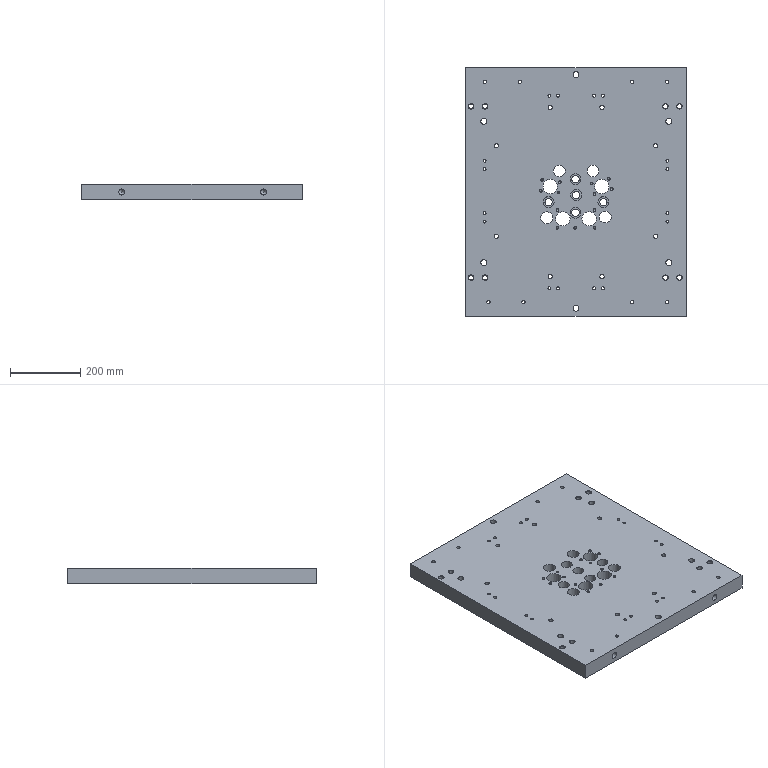Part | NX | features solid 2 | 1 solid | 450 faces | box 630 x 710 x 45 mm | volume 18865947 mm3 | cone 196 | cylinder 187 | plane 67 | commonest cylinder face diameters 10 x40 8.5 x36 10.3 x30 6.8 x23 12 x8 14 x8